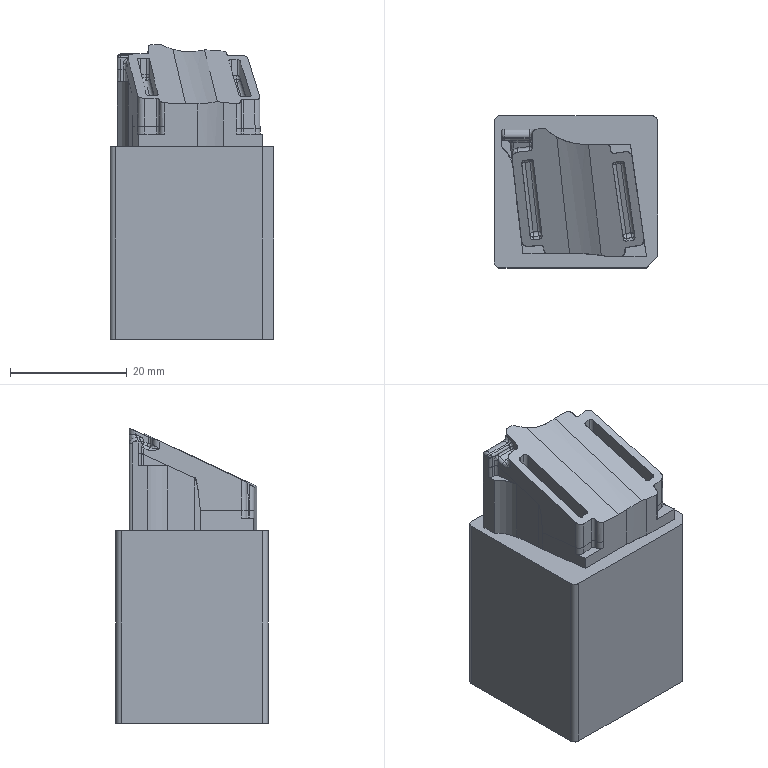CAM job | NX | 3-axis milling | part box 28 x 26 x 50.455 mm | stock box 28 x 26 x 50.455 mm
Tools:
number,name,description,diameter,corner_radius,flute_length,length,flutes
0,D6,Milling Tool-5 Parameters,6.0,0.0,50.0,75.0,2
0,1,Milling Tool-5 Parameters,1.0,0.0,50.0,75.0,2
0,MILL_2,Milling Tool-5 Parameters,0.5,0.0,50.0,75.0,2
0,D0.5,Milling Tool-5 Parameters,0.5,0.0,50.0,75.0,2
0,D0.8R0.4,Milling Tool-5 Parameters,0.8,0.4,50.0,75.0,2
0,D6R3,Milling Tool-5 Parameters,6.0,3.0,50.0,75.0,2
Operations:
program,operation,operation_type,tool,method,geometry_group,spindle_rpm,surface_speed,feed_per_tooth,feed_cut,feed_plunge,cut_length_mm,path_length_mm,cut_time_min,machine_time_min
A1,CAVITY_MILL,CavityMilling,D6,METHOD,WORKPIECE,0.0,0.0,0.0,250.0,100.0,14213.006,16014.772,56.852,57.032
A2,CAVITY_MILL_COPY,CavityMilling,1,METHOD,WORKPIECE,0.0,0.0,0.0,250.0,100.0,2796.443,3717.047,11.186,11.278
A3,CAVITY_MILL_COPY_COPY,CavityMilling,MILL_2,METHOD,WORKPIECE,0.0,0.0,0.0,250.0,100.0,587.683,727.209,2.351,2.365
A4,CAVITY_MILL_COPY_COPY_COPY,CavityMilling,D6,METHOD,WORKPIECE,0.0,0.0,0.0,250.0,100.0,117.151,171.461,0.4686,0.474
A5,ZLEVEL_PROFILE_COPY,ZLevelMilling,D0.5,METHOD,WORKPIECE,0.0,0.0,0.0,250.0,100.0,10964.499,11583.252,43.858,43.92
A6,ZLEVEL_PROFILE,ZLevelMilling,D0.8R0.4,METHOD,WORKPIECE,0.0,0.0,0.0,250.0,100.0,2564.919,2825.577,10.26,10.286
A7,CONTOUR_AREA,SurfaceContour,D6R3,METHOD,WORKPIECE,0.0,0.0,0.0,250.0,100.0,4813.728,4864.157,19.255,19.26
A8,CONTOUR_AREA_1,SurfaceContour,D0.8R0.4,METHOD,WORKPIECE,0.0,0.0,0.0,250.0,100.0,316.528,356.932,1.266,1.27
A9,ZLEVEL_PROFILE_1,ZLevelMilling,D0.8R0.4,METHOD,WORKPIECE,0.0,0.0,0.0,250.0,100.0,459.735,520.514,1.839,1.845